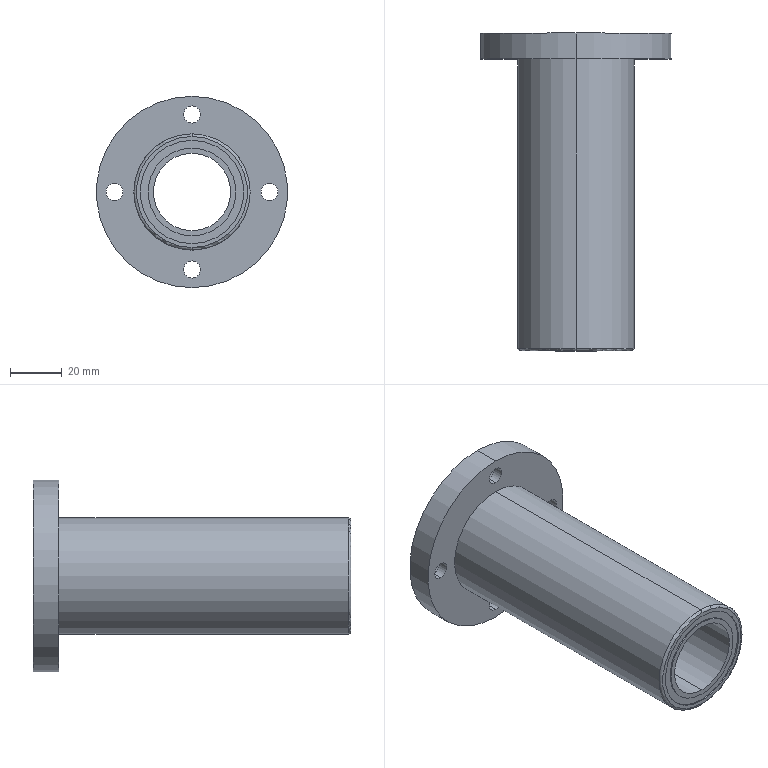Part | STEP file | LMF30LUU | 1 solid | 43 faces | box 74 x 123 x 74 mm | volume 132378 mm3 | cylinder 30 | plane 11 | torus 2 | commonest cylinder face diameters 6.6 x8 11 x8 34 x4 40 x4 30 x2 45 x2